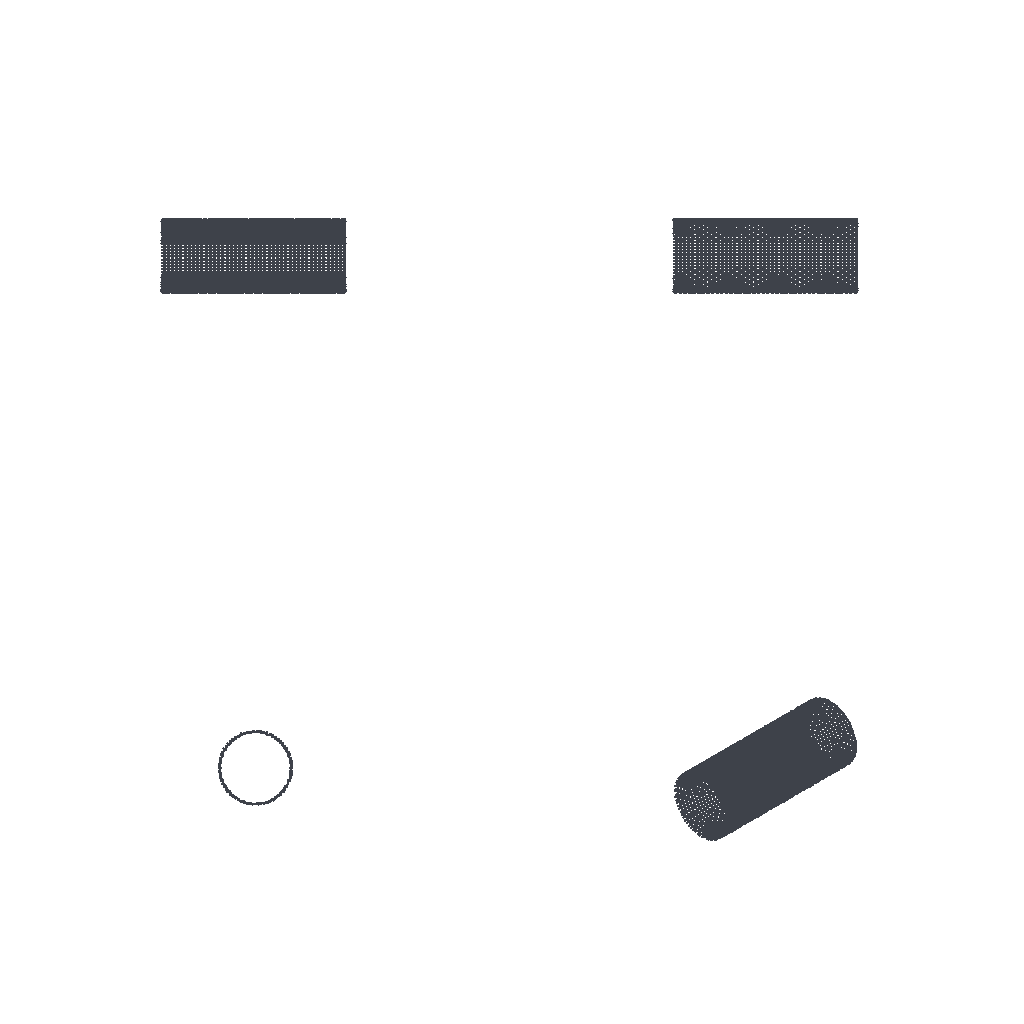Simulation study | abaqus
Set-up summary:
category,name,step,type,value,unit,region
solver,abaqus
solver,version,,,Abaqus/Explicit 2020
units,not stated in the deck,,not stated
analysis,deck,,transient,transient
load_step,Step-ya,Step-ya,transient,nlgeom=True
load_step,Step-1,Step-1,transient,nlgeom=True
contact,interactions,,,general=1 pairs=0 ties=0
load_step,requested,,,2
mesh,nodes,,,41311
mesh,elements,,,40572
element_type,R3D4,,rigid,12500
element_type,T3D2,,truss,28072
load,load commands in deck,,count,4
bc,support commands in deck,,count,26
material,MATERIAL-1,,in results
check,setup vs results,,match,"per instance, exact: element labels, types and connectivity; labels of the nodes the elements use; coordinates of those nodes at SINGLE_PRECISION in 116 of 116 instance(s)"
Abaqus input file, long lists of numbers shortened:
*Heading
** Job name: Job-3 Model name: Model-1-Copy-Copy
** Generated by: Abaqus/CAE 2020
*Preprint, echo=NO, model=NO, history=NO, contact=NO
**
** PARTS
**
*Part, name=jing-1
*Node
      1,         8.75,  0.2408,           0.
      2,        9.625,  0.2408,           0.
** (239 more lines like these left out)
*Element, type=T3D2
 1,  1, 22
 2, 22, 23
** (238 more lines like these left out)
*Nset, nset=Set-1, generate
   1,  241,    1
*Elset, elset=Set-1, generate
   1,  240,    1
** Section: Section-2
*Solid Section, elset=Set-1, material=Material-1
0.0045,
*End Part
**
*Part, name=jing-2
*Node
      1,   23.642,  0.2408,           0.
      2,   24.517,  0.2408,           0.
** (208 more lines like these left out)
*Element, type=T3D2
 1,  1, 31
 2, 31, 32
** (198 more lines like these left out)
*Nset, nset=Set-1, generate
   1,  210,    1
*Elset, elset=Set-1, generate
   1,  200,    1
** Section: Section-2
*Solid Section, elset=Set-1, material=Material-1
0.0045,
*End Part
**
*Part, name=qiao
*Node
      1,          25.,           0.,           0.
      2,   24.8,           0.,           0.
** (6424 more lines like these left out)
*Element, type=R3D4
   1,    1,    2,  128,  127
   2,    2,    3,  129,  128
** (6248 more lines like these left out)
*Node
   6427,         12.5,          -5.,           0.
*Nset, nset=qiao-RefPt_, internal
6427,
*Elset, elset=qiao, generate
    1,  6250,     1
*End Part
**
*Part, name=wei-1
*Node
      1,           0.,   3.803,           0.
      2, -0.5904,   3.752,           0.
** (286 more lines like these left out)
*Element, type=T3D2
1,  2, 37
2, 37, 38
** (286 more lines like these left out)
*Nset, nset=Set-1, generate
   1,  288,    1
*Elset, elset=Set-1, generate
   1,  288,    1
** Section: Section-1
*Solid Section, elset=Set-1, material=Material-1
0.003,
*End Part
**
**
** ASSEMBLY
**
*Assembly, name=Assembly
**
*Instance, name=jing-1-1, part=jing-1
          0.,          3.2,           0.
*End Instance
**
*Instance, name=jing-1-1-rad-2, part=jing-1
          0., 3.149, 0.5714
          0., 3.149, 0.5714, 1., 3.149, 0.5714, 10.286
*End Instance
**
*Instance, name=jing-1-1-rad-3, part=jing-1
          0., 2.996, 1.124
          0., 2.996, 1.124, 1., 2.996, 1.124, 20.571
*End Instance
**
*Instance, name=jing-1-1-rad-4, part=jing-1
          0., 2.747, 1.641
          0., 2.747, 1.641, 1., 2.747, 1.641, 30.857
*End Instance
**
*Instance, name=jing-1-1-rad-5, part=jing-1
          0., 2.41, 2.105
          0., 2.41, 2.105, 1., 2.41, 2.105, 41.143
*End Instance
**
*Instance, name=jing-1-1-rad-6, part=jing-1
          0., 1.995, 2.502
          0., 1.995, 2.502, 1., 1.995, 2.502, 51.429
*End Instance
**
*Instance, name=jing-1-1-rad-7, part=jing-1
          0., 1.516, 2.818
          0., 1.516, 2.818, 1., 1.516, 2.818, 61.714
*End Instance
**
*Instance, name=jing-1-1-rad-8, part=jing-1
          0., 0.9889, 3.043
          0., 0.9889, 3.043, 1., 0.9889, 3.043, 72.
*End Instance
**
*Instance, name=jing-1-1-rad-9, part=jing-1
          0., 0.4295, 3.171
          0., 0.4295, 3.171, 1., 0.4295, 3.171, 82.286
*End Instance
**
*Instance, name=jing-1-1-rad-10, part=jing-1
          0., -0.1436, 3.197
          0., -0.1436, 3.197, 1., -0.1436, 3.197, 92.571
*End Instance
**
*Instance, name=jing-1-1-rad-11, part=jing-1
          0., -0.7121, 3.12
          0., -0.7121, 3.12, 1., -0.7121, 3.12, 102.857
*End Instance
**
*Instance, name=jing-1-1-rad-12, part=jing-1
          0., -1.258, 2.942
          0., -1.258, 2.942, 1., -1.258, 2.942, 113.143
*End Instance
**
*Instance, name=jing-1-1-rad-13, part=jing-1
          0., -1.763, 2.671
          0., -1.763, 2.671, 1., -1.763, 2.671, 123.429
*End Instance
**
*Instance, name=jing-1-1-rad-14, part=jing-1
          0., -2.211, 2.313
          0., -2.211, 2.313, 1., -2.211, 2.313, 133.714
*End Instance
**
*Instance, name=jing-1-1-rad-15, part=jing-1
          0., -2.589, 1.881
          0., -2.589, 1.881, 1., -2.589, 1.881, 144.
*End Instance
**
*Instance, name=jing-1-1-rad-16, part=jing-1
          0., -2.883, 1.388
          0., -2.883, 1.388, 1., -2.883, 1.388, 154.286
*End Instance
**
*Instance, name=jing-1-1-rad-17, part=jing-1
          0., -3.085, 0.8513
          0., -3.085, 0.8513, 1., -3.085, 0.8513, 164.571
*End Instance
**
*Instance, name=jing-1-1-rad-18, part=jing-1
          0., -3.187, 0.2868
          0., -3.187, 0.2868, 1., -3.187, 0.2868, 174.857
*End Instance
**
*Instance, name=jing-1-1-rad-19, part=jing-1
          0., -3.187, -0.2868
          0., -3.187, -0.2868, 1., -3.187, -0.2868, 185.143
*End Instance
**
*Instance, name=jing-1-1-rad-20, part=jing-1
          0., -3.085, -0.8513
          0., -3.085, -0.8513, 1., -3.085, -0.8513, 195.429
*End Instance
**
*Instance, name=jing-1-1-rad-21, part=jing-1
          0., -2.883, -1.388
          0., -2.883, -1.388, 1., -2.883, -1.388, 205.714
*End Instance
**
*Instance, name=jing-1-1-rad-22, part=jing-1
          0., -2.589, -1.881
          0., -2.589, -1.881, 1., -2.589, -1.881, 216.
*End Instance
**
*Instance, name=jing-1-1-rad-23, part=jing-1
          0., -2.211, -2.313
          0., -2.211, -2.313, 1., -2.211, -2.313, 226.286
*End Instance
**
*Instance, name=jing-1-1-rad-24, part=jing-1
          0., -1.763, -2.671
          0., -1.763, -2.671, 1., -1.763, -2.671, 236.571
*End Instance
**
*Instance, name=jing-1-1-rad-25, part=jing-1
          0., -1.258, -2.942
          0., -1.258, -2.942, -1., -1.258, -2.942, 113.143
*End Instance
**
*Instance, name=jing-1-1-rad-26, part=jing-1
          0., -0.7121, -3.12
          0., -0.7121, -3.12, -1., -0.7121, -3.12, 102.857
*End Instance
**
*Instance, name=jing-1-1-rad-27, part=jing-1
          0., -0.1436, -3.197
          0., -0.1436, -3.197, -1., -0.1436, -3.197, 92.571
*End Instance
**
*Instance, name=jing-1-1-rad-28, part=jing-1
          0., 0.4295, -3.171
          0., 0.4295, -3.171, -1., 0.4295, -3.171, 82.286
*End Instance
**
*Instance, name=jing-1-1-rad-29, part=jing-1
          0., 0.9889, -3.043
          0., 0.9889, -3.043, -1., 0.9889, -3.043, 72.
*End Instance
**
*Instance, name=jing-1-1-rad-30, part=jing-1
          0., 1.516, -2.818
          0., 1.516, -2.818, -1., 1.516, -2.818, 61.714
*End Instance
**
*Instance, name=jing-1-1-rad-31, part=jing-1
          0., 1.995, -2.502
          0., 1.995, -2.502, -1., 1.995, -2.502, 51.429
*End Instance
**
*Instance, name=jing-1-1-rad-32, part=jing-1
          0., 2.41, -2.105
          0., 2.41, -2.105, -1., 2.41, -2.105, 41.143
*End Instance
**
*Instance, name=jing-1-1-rad-33, part=jing-1
          0., 2.747, -1.641
          0., 2.747, -1.641, -1., 2.747, -1.641, 30.857
*End Instance
**
*Instance, name=jing-1-1-rad-34, part=jing-1
          0., 2.996, -1.124
          0., 2.996, -1.124, -1., 2.996, -1.124, 20.571
*End Instance
**
*Instance, name=jing-1-1-rad-35, part=jing-1
          0., 3.149, -0.5714
          0., 3.149, -0.5714, -1., 3.149, -0.5714, 10.286
*End Instance
**
*Instance, name=jing-2-1, part=jing-2
          0., 3.188, 0.2789
          0., 3.188, 0.2789, 1., 3.188, 0.2789, 5.
*End Instance
**
*Instance, name=jing-2-1-rad-2, part=jing-2
          0., 3.087, 0.8436
          0., 3.087, 0.8436, 1., 3.087, 0.8436, 15.286
*End Instance
**
*Instance, name=jing-2-1-rad-3, part=jing-2
          0., 2.887, 1.381
          0., 2.887, 1.381, 1., 2.887, 1.381, 25.571
*End Instance
**
*Instance, name=jing-2-1-rad-4, part=jing-2
          0., 2.594, 1.874
          0., 2.594, 1.874, 1., 2.594, 1.874, 35.857
*End Instance
**
*Instance, name=jing-2-1-rad-5, part=jing-2
          0., 2.217, 2.307
          0., 2.217, 2.307, 1., 2.217, 2.307, 46.143
*End Instance
**
*Instance, name=jing-2-1-rad-6, part=jing-2
          0., 1.77, 2.666
          0., 1.77, 2.666, 1., 1.77, 2.666, 56.429
*End Instance
**
*Instance, name=jing-2-1-rad-7, part=jing-2
          0., 1.265, 2.939
          0., 1.265, 2.939, 1., 1.265, 2.939, 66.714
*End Instance
**
*Instance, name=jing-2-1-rad-8, part=jing-2
          0., 0.7198, 3.118
          0., 0.7198, 3.118, 1., 0.7198, 3.118, 77.
*End Instance
**
*Instance, name=jing-2-1-rad-9, part=jing-2
          0., 0.1515, 3.196
          0., 0.1515, 3.196, 1., 0.1515, 3.196, 87.286
*End Instance
**
*Instance, name=jing-2-1-rad-10, part=jing-2
          0., -0.4216, 3.172
          0., -0.4216, 3.172, 1., -0.4216, 3.172, 97.571
*End Instance
**
*Instance, name=jing-2-1-rad-11, part=jing-2
          0., -0.9813, 3.046
          0., -0.9813, 3.046, 1., -0.9813, 3.046, 107.857
*End Instance
**
*Instance, name=jing-2-1-rad-12, part=jing-2
          0., -1.509, 2.822
          0., -1.509, 2.822, 1., -1.509, 2.822, 118.143
*End Instance
**
*Instance, name=jing-2-1-rad-13, part=jing-2
          0., -1.989, 2.507
          0., -1.989, 2.507, 1., -1.989, 2.507, 128.429
*End Instance
**
*Instance, name=jing-2-1-rad-14, part=jing-2
          0., -2.405, 2.111
          0., -2.405, 2.111, 1., -2.405, 2.111, 138.714
*End Instance
**
*Instance, name=jing-2-1-rad-15, part=jing-2
          0., -2.743, 1.648
          0., -2.743, 1.648, 1., -2.743, 1.648, 149.
*End Instance
**
*Instance, name=jing-2-1-rad-16, part=jing-2
          0., -2.993, 1.132
          0., -2.993, 1.132, 1., -2.993, 1.132, 159.286
*End Instance
**
*Instance, name=jing-2-1-rad-17, part=jing-2
          0., -3.147, 0.5792
          0., -3.147, 0.5792, 1., -3.147, 0.5792, 169.571
*End Instance
**
*Instance, name=jing-2-1-rad-18, part=jing-2
          0., -3.2, 0.007979
          0., -3.2, 0.007979, 1., -3.2, 0.007979, 179.857
*End Instance
**
*Instance, name=jing-2-1-rad-19, part=jing-2
          0., -3.15, -0.5635
          0., -3.15, -0.5635, 1., -3.15, -0.5635, 190.143
*End Instance
**
*Instance, name=jing-2-1-rad-20, part=jing-2
          0., -2.999, -1.117
          0., -2.999, -1.117, 1., -2.999, -1.117, 200.429
*End Instance
**
*Instance, name=jing-2-1-rad-21, part=jing-2
          0., -2.751, -1.634
          0., -2.751, -1.634, 1., -2.751, -1.634, 210.714
*End Instance
**
*Instance, name=jing-2-1-rad-22, part=jing-2
          0., -2.415, -2.099
          0., -2.415, -2.099, 1., -2.415, -2.099, 221.
*End Instance
**
*Instance, name=jing-2-1-rad-23, part=jing-2
          0., -2.001, -2.497
          0., -2.001, -2.497, 1., -2.001, -2.497, 231.286
*End Instance
**
*Instance, name=jing-2-1-rad-24, part=jing-2
          0., -1.523, -2.814
          0., -1.523, -2.814, -1., -1.523, -2.814, 118.429
*End Instance
**
*Instance, name=jing-2-1-rad-25, part=jing-2
          0., -0.9964, -3.041
          0., -0.9964, -3.041, -1., -0.9964, -3.041, 108.143
*End Instance
**
*Instance, name=jing-2-1-rad-26, part=jing-2
          0., -0.4375, -3.17
          0., -0.4375, -3.17, -1., -0.4375, -3.17, 97.857
*End Instance
**
*Instance, name=jing-2-1-rad-27, part=jing-2
          0., 0.1356, -3.197
          0., 0.1356, -3.197, -1., 0.1356, -3.197, 87.571
*End Instance
**
*Instance, name=jing-2-1-rad-28, part=jing-2
          0., 0.7043, -3.122
          0., 0.7043, -3.122, -1., 0.7043, -3.122, 77.286
*End Instance
**
*Instance, name=jing-2-1-rad-29, part=jing-2
          0., 1.25, -2.946
          0., 1.25, -2.946, -1., 1.25, -2.946, 67.
*End Instance
**
*Instance, name=jing-2-1-rad-30, part=jing-2
          0., 1.756, -2.675
          0., 1.756, -2.675, -1., 1.756, -2.675, 56.714
*End Instance
**
*Instance, name=jing-2-1-rad-31, part=jing-2
          0., 2.206, -2.318
          0., 2.206, -2.318, -1., 2.206, -2.318, 46.429
*End Instance
**
*Instance, name=jing-2-1-rad-32, part=jing-2
          0., 2.584, -1.887
          0., 2.584, -1.887, -1., 2.584, -1.887, 36.143
*End Instance
**
*Instance, name=jing-2-1-rad-33, part=jing-2
          0., 2.88, -1.396
          0., 2.88, -1.396, -1., 2.88, -1.396, 25.857
*End Instance
**
*Instance, name=jing-2-1-rad-34, part=jing-2
          0., 3.083, -0.859
          0., 3.083, -0.859, -1., 3.083, -0.859, 15.571
*End Instance
**
*Instance, name=jing-2-1-rad-35, part=jing-2
          0., 3.186, -0.2948
          0., 3.186, -0.2948, -1., 3.186, -0.2948, 5.286
*End Instance
**
*Instance, name=wei-1-1, part=wei-1
          9., -0.3951, -0.06959
          9., -0.3951, -0.06959, 9.07, 0.6, 8.23284404274927e-07, 90.279
*End Instance
**
*Instance, name=wei-1-1-lin-2-1, part=wei-1
         9.4, -0.3951, -0.06959
         9.4, -0.3951, -0.06959, 9.47, 0.6, 8.23284404274927e-07, 90.279
*End Instance
**
*Instance, name=wei-1-1-lin-3-1, part=wei-1
         9.8, -0.3951, -0.06959
         9.8, -0.3951, -0.06959, 9.87, 0.6, 8.23284404274927e-07, 90.279
*End Instance
**
*Instance, name=wei-1-1-lin-4-1, part=wei-1
        10.2, -0.3951, -0.06959
        10.2, -0.3951, -0.06959, 10.27, 0.6, 8.23284404274927e-07, 90.279
*End Instance
**
*Instance, name=wei-1-1-lin-5-1, part=wei-1
        10.6, -0.3951, -0.06959
        10.6, -0.3951, -0.06959, 10.67, 0.6, 8.23284404274927e-07, 90.279
*End Instance
**
*Instance, name=wei-1-1-lin-6-1, part=wei-1
         11., -0.3951, -0.06959
         11., -0.3951, -0.06959, 11.07, 0.6, 8.23284404274927e-07, 90.279
*End Instance
**
*Instance, name=wei-1-1-lin-7-1, part=wei-1
        11.4, -0.3951, -0.06959
        11.4, -0.3951, -0.06959, 11.47, 0.6, 8.23284404274927e-07, 90.279
*End Instance
**
*Instance, name=wei-1-1-lin-8-1, part=wei-1
        11.8, -0.3951, -0.06959
        11.8, -0.3951, -0.06959, 11.87, 0.6, 8.23284404274927e-07, 90.279
*End Instance
**
*Instance, name=wei-1-1-lin-9-1, part=wei-1
        12.2, -0.3951, -0.06959
        12.2, -0.3951, -0.06959, 12.27, 0.6, 8.23284404274927e-07, 90.279
*End Instance
**
*Instance, name=wei-1-1-lin-10-1, part=wei-1
        12.6, -0.3951, -0.06959
        12.6, -0.3951, -0.06959, 12.67, 0.6, 8.23284404274927e-07, 90.279
*End Instance
**
*Instance, name=wei-1-1-lin-11-1, part=wei-1
         13., -0.3951, -0.06959
         13., -0.3951, -0.06959, 13.07, 0.6, 8.23284404274927e-07, 90.279
*End Instance
**
*Instance, name=wei-1-1-lin-12-1, part=wei-1
        13.4, -0.3951, -0.06959
        13.4, -0.3951, -0.06959, 13.47, 0.6, 8.23284404274927e-07, 90.279
*End Instance
**
*Instance, name=wei-1-1-lin-13-1, part=wei-1
        13.8, -0.3951, -0.06959
        13.8, -0.3951, -0.06959, 13.87, 0.6, 8.23284404274927e-07, 90.279
*End Instance
**
*Instance, name=wei-1-1-lin-14-1, part=wei-1
        14.2, -0.3951, -0.06959
        14.2, -0.3951, -0.06959, 14.27, 0.6, 8.23284404274927e-07, 90.279
*End Instance
**
*Instance, name=wei-1-1-lin-15-1, part=wei-1
        14.6, -0.3951, -0.06959
        14.6, -0.3951, -0.06959, 14.67, 0.6, 8.23284404274927e-07, 90.279
*End Instance
**
*Instance, name=wei-1-1-lin-16-1, part=wei-1
         15., -0.3951, -0.06959
         15., -0.3951, -0.06959, 15.07, 0.6, 8.23284404274927e-07, 90.279
*End Instance
**
*Instance, name=wei-1-1-lin-17-1, part=wei-1
        15.4, -0.3951, -0.06959
        15.4, -0.3951, -0.06959, 15.47, 0.6, 8.23284404274927e-07, 90.279
*End Instance
**
*Instance, name=wei-1-1-lin-18-1, part=wei-1
        15.8, -0.3951, -0.06959
        15.8, -0.3951, -0.06959, 15.87, 0.6, 8.23284404274927e-07, 90.279
*End Instance
**
*Instance, name=wei-1-1-lin-19-1, part=wei-1
        16.2, -0.3951, -0.06959
        16.2, -0.3951, -0.06959, 16.27, 0.6, 8.23284404274927e-07, 90.279
*End Instance
**
*Instance, name=wei-1-1-lin-20-1, part=wei-1
        16.6, -0.3951, -0.06959
        16.6, -0.3951, -0.06959, 16.67, 0.6, 8.23284404274927e-07, 90.279
*End Instance
**
*Instance, name=wei-1-1-lin-21-1, part=wei-1
         17., -0.3951, -0.06959
         17., -0.3951, -0.06959, 17.07, 0.6, 8.23284404274927e-07, 90.279
*End Instance
**
*Instance, name=wei-1-1-lin-22-1, part=wei-1
        17.4, -0.3951, -0.06959
        17.4, -0.3951, -0.06959, 17.47, 0.6, 8.23284404274927e-07, 90.279
*End Instance
**
*Instance, name=wei-1-1-lin-23-1, part=wei-1
        17.8, -0.3951, -0.06959
        17.8, -0.3951, -0.06959, 17.87, 0.6, 8.23284404274927e-07, 90.279
*End Instance
**
*Instance, name=wei-1-1-lin-24-1, part=wei-1
        18.2, -0.3951, -0.06959
        18.2, -0.3951, -0.06959, 18.27, 0.6, 8.23284404274927e-07, 90.279
*End Instance
**
*Instance, name=wei-1-1-lin-25-1, part=wei-1
        18.6, -0.3951, -0.06959
        18.6, -0.3951, -0.06959, 18.67, 0.6, 8.23284404274927e-07, 90.279
*End Instance
**
*Instance, name=wei-1-1-lin-26-1, part=wei-1
         19., -0.3951, -0.06959
         19., -0.3951, -0.06959, 19.07, 0.6, 8.23284404274927e-07, 90.279
*End Instance
**
*Instance, name=wei-1-1-lin-27-1, part=wei-1
        19.4, -0.3951, -0.06959
        19.4, -0.3951, -0.06959, 19.47, 0.6, 8.23284404274927e-07, 90.279
*End Instance
**
*Instance, name=wei-1-1-lin-28-1, part=wei-1
        19.8, -0.3951, -0.06959
        19.8, -0.3951, -0.06959, 19.87, 0.6, 8.23284404274927e-07, 90.279
*End Instance
**
*Instance, name=wei-1-1-lin-29-1, part=wei-1
        20.2, -0.3951, -0.06959
        20.2, -0.3951, -0.06959, 20.27, 0.6, 8.23284404274927e-07, 90.279
*End Instance
**
*Instance, name=wei-1-1-lin-30-1, part=wei-1
        20.6, -0.3951, -0.06959
        20.6, -0.3951, -0.06959, 20.67, 0.6, 8.23284404274927e-07, 90.279
*End Instance
**
*Instance, name=wei-1-1-lin-31-1, part=wei-1
         21., -0.3951, -0.06959
         21., -0.3951, -0.06959, 21.07, 0.6, 8.23284404274927e-07, 90.279
*End Instance
**
*Instance, name=wei-1-1-lin-32-1, part=wei-1
        21.4, -0.3951, -0.06959
        21.4, -0.3951, -0.06959, 21.47, 0.6, 8.23284404274927e-07, 90.279
*End Instance
**
*Instance, name=wei-1-1-lin-33-1, part=wei-1
        21.8, -0.3951, -0.06959
        21.8, -0.3951, -0.06959, 21.87, 0.6, 8.23284404274927e-07, 90.279
*End Instance
**
*Instance, name=wei-1-1-lin-34-1, part=wei-1
        22.2, -0.3951, -0.06959
        22.2, -0.3951, -0.06959, 22.27, 0.6, 8.23284404274927e-07, 90.279
*End Instance
**
*Instance, name=wei-1-1-lin-35-1, part=wei-1
        22.6, -0.3951, -0.06959
        22.6, -0.3951, -0.06959, 22.67, 0.6, 8.23284404274927e-07, 90.279
*End Instance
**
*Instance, name=wei-1-1-lin-36-1, part=wei-1
         23., -0.3951, -0.06959
         23., -0.3951, -0.06959, 23.07, 0.6, 8.23284404274927e-07, 90.279
*End Instance
**
*Instance, name=wei-1-1-lin-37-1, part=wei-1
        23.4, -0.3951, -0.06959
        23.4, -0.3951, -0.06959, 23.47, 0.6, 8.23284404274927e-07, 90.279
*End Instance
**
*Instance, name=wei-1-1-lin-38-1, part=wei-1
        23.8, -0.3951, -0.06959
        23.8, -0.3951, -0.06959, 23.87, 0.6, 8.23284404274927e-07, 90.279
*End Instance
**
*Instance, name=wei-1-1-lin-39-1, part=wei-1
        24.2, -0.3951, -0.06959
        24.2, -0.3951, -0.06959, 24.27, 0.6, 8.23284404274927e-07, 90.279
*End Instance
**
*Instance, name=wei-1-1-lin-40-1, part=wei-1
        24.6, -0.3951, -0.06959
        24.6, -0.3951, -0.06959, 24.67, 0.6, 8.23284404274927e-07, 90.279
*End Instance
**
*Instance, name=wei-1-1-lin-41-1, part=wei-1
         25., -0.3951, -0.06959
         25., -0.3951, -0.06959, 25.07, 0.6, 8.23284404274927e-07, 90.279
*End Instance
**
*Instance, name=wei-1-1-lin-42-1, part=wei-1
        25.4, -0.3951, -0.06959
        25.4, -0.3951, -0.06959, 25.47, 0.6, 8.23284404274927e-07, 90.279
*End Instance
**
*Instance, name=wei-1-1-lin-43-1, part=wei-1
        25.8, -0.3951, -0.06959
        25.8, -0.3951, -0.06959, 25.87, 0.6, 8.23284404274927e-07, 90.279
*End Instance
**
*Instance, name=wei-1-1-lin-44-1, part=wei-1
        26.2, -0.3951, -0.06959
        26.2, -0.3951, -0.06959, 26.27, 0.6, 8.23284404274927e-07, 90.279
*End Instance
**
*Instance, name=qiao-1, part=qiao
        5.25,     4.962,     3.56
*End Instance
**
*Instance, name=qiao-1-lin-2-1, part=qiao
        5.25,     4.962,    -3.59
*End Instance
**
*Nset, nset=Set-1, instance=jing-1-1
  20,  21, 231, 232, 233, 234, 235, 236, 237, 238, 239, 240, 241
*Nset, nset=Set-1, instance=jing-1-1-rad-2
  20,  21, 231, 232, 233, 234, 235, 236, 237, 238, 239, 240, 241
*Nset, nset=Set-1, instance=jing-1-1-rad-3
  20,  21, 231, 232, 233, 234, 235, 236, 237, 238, 239, 240, 241
*Nset, nset=Set-1, instance=jing-1-1-rad-5
  20,  21, 231, 232, 233, 234, 235, 236, 237, 238, 239, 240, 241
*Nset, nset=Set-1, instance=jing-1-1-rad-9
  20,  21, 231, 232, 233, 234, 235, 236, 237, 238, 239, 240, 241
*Nset, nset=Set-1, instance=jing-1-1-rad-25
  20,  21, 231, 232, 233, 234, 235, 236, 237, 238, 239, 240, 241
*Nset, nset=Set-1, instance=jing-2-1-rad-22
  29,  30, 202, 203, 204, 205, 206, 207, 208, 209, 210
*Nset, nset=Set-1, instance=jing-2-1-rad-6
  29,  30, 202, 203, 204, 205, 206, 207, 208, 209, 210
*Nset, nset=Set-1, instance=jing-1-1-rad-17
  20,  21, 231, 232, 233, 234, 235, 236, 237, 238, 239, 240, 241
*Nset, nset=Set-1, instance=jing-1-1-rad-33
  20,  21, 231, 232, 233, 234, 235, 236, 237, 238, 239, 240, 241
*Nset, nset=Set-1, instance=jing-2-1-rad-30
  29,  30, 202, 203, 204, 205, 206, 207, 208, 209, 210
*Nset, nset=Set-1, instance=jing-2-1-rad-14
  29,  30, 202, 203, 204, 205, 206, 207, 208, 209, 210
*Nset, nset=Set-1, instance=wei-1-1-lin-43-1, generate
   1,  288,    1
*Nset, nset=Set-1, instance=jing-1-1-rad-13
  20,  21, 231, 232, 233, 234, 235, 236, 237, 238, 239, 240, 241
*Nset, nset=Set-1, instance=jing-1-1-rad-29
  20,  21, 231, 232, 233, 234, 235, 236, 237, 238, 239, 240, 241
*Nset, nset=Set-1, instance=jing-2-1-rad-26
  29,  30, 202, 203, 204, 205, 206, 207, 208, 209, 210
*Nset, nset=Set-1, instance=jing-2-1-rad-10
  29,  30, 202, 203, 204, 205, 206, 207, 208, 209, 210
*Nset, nset=Set-1, instance=jing-1-1-rad-21
  20,  21, 231, 232, 233, 234, 235, 236, 237, 238, 239, 240, 241
*Nset, nset=Set-1, instance=jing-2-1-rad-2
  29,  30, 202, 203, 204, 205, 206, 207, 208, 209, 210
*Nset, nset=Set-1, instance=jing-2-1-rad-34
  29,  30, 202, 203, 204, 205, 206, 207, 208, 209, 210
*Nset, nset=Set-1, instance=jing-2-1-rad-18
  29,  30, 202, 203, 204, 205, 206, 207, 208, 209, 210
*Nset, nset=Set-1, instance=jing-1-1-rad-7
  20,  21, 231, 232, 233, 234, 235, 236, 237, 238, 239, 240, 241
*Nset, nset=Set-1, instance=jing-1-1-rad-11
  20,  21, 231, 232, 233, 234, 235, 236, 237, 238, 239, 240, 241
*Nset, nset=Set-1, instance=jing-1-1-rad-27
  20,  21, 231, 232, 233, 234, 235, 236, 237, 238, 239, 240, 241
*Nset, nset=Set-1, instance=jing-2-1-rad-24
  29,  30, 202, 203, 204, 205, 206, 207, 208, 209, 210
*Nset, nset=Set-1, instance=jing-2-1-rad-8
  29,  30, 202, 203, 204, 205, 206, 207, 208, 209, 210
*Nset, nset=Set-1, instance=jing-1-1-rad-19
  20,  21, 231, 232, 233, 234, 235, 236, 237, 238, 239, 240, 241
*Nset, nset=Set-1, instance=jing-1-1-rad-35
  20,  21, 231, 232, 233, 234, 235, 236, 237, 238, 239, 240, 241
*Nset, nset=Set-1, instance=jing-2-1-rad-32
  29,  30, 202, 203, 204, 205, 206, 207, 208, 209, 210
*Nset, nset=Set-1, instance=jing-2-1-rad-16
  29,  30, 202, 203, 204, 205, 206, 207, 208, 209, 210
*Nset, nset=Set-1, instance=jing-1-1-rad-15
  20,  21, 231, 232, 233, 234, 235, 236, 237, 238, 239, 240, 241
*Nset, nset=Set-1, instance=jing-1-1-rad-31
  20,  21, 231, 232, 233, 234, 235, 236, 237, 238, 239, 240, 241
*Nset, nset=Set-1, instance=jing-2-1-rad-28
  29,  30, 202, 203, 204, 205, 206, 207, 208, 209, 210
*Nset, nset=Set-1, instance=jing-2-1-rad-12
  29,  30, 202, 203, 204, 205, 206, 207, 208, 209, 210
*Nset, nset=Set-1, instance=jing-1-1-rad-23
  20,  21, 231, 232, 233, 234, 235, 236, 237, 238, 239, 240, 241
*Nset, nset=Set-1, instance=jing-2-1-rad-4
  29,  30, 202, 203, 204, 205, 206, 207, 208, 209, 210
*Nset, nset=Set-1, instance=jing-2-1-rad-20
  29,  30, 202, 203, 204, 205, 206, 207, 208, 209, 210
*Nset, nset=Set-1, instance=jing-1-1-rad-4
  20,  21, 231, 232, 233, 234, 235, 236, 237, 238, 239, 240, 241
*Nset, nset=Set-1, instance=jing-1-1-rad-6
  20,  21, 231, 232, 233, 234, 235, 236, 237, 238, 239, 240, 241
*Nset, nset=Set-1, instance=jing-1-1-rad-10
  20,  21, 231, 232, 233, 234, 235, 236, 237, 238, 239, 240, 241
*Nset, nset=Set-1, instance=jing-1-1-rad-26
  20,  21, 231, 232, 233, 234, 235, 236, 237, 238, 239, 240, 241
*Nset, nset=Set-1, instance=jing-2-1-rad-23
  29,  30, 202, 203, 204, 205, 206, 207, 208, 209, 210
*Nset, nset=Set-1, instance=jing-2-1-rad-7
  29,  30, 202, 203, 204, 205, 206, 207, 208, 209, 210
*Nset, nset=Set-1, instance=jing-1-1-rad-18
  20,  21, 231, 232, 233, 234, 235, 236, 237, 238, 239, 240, 241
*Nset, nset=Set-1, instance=jing-1-1-rad-34
  20,  21, 231, 232, 233, 234, 235, 236, 237, 238, 239, 240, 241
*Nset, nset=Set-1, instance=jing-2-1-rad-31
  29,  30, 202, 203, 204, 205, 206, 207, 208, 209, 210
*Nset, nset=Set-1, instance=jing-2-1-rad-15
  29,  30, 202, 203, 204, 205, 206, 207, 208, 209, 210
*Nset, nset=Set-1, instance=wei-1-1-lin-44-1, generate
   1,  288,    1
*Nset, nset=Set-1, instance=jing-1-1-rad-14
  20,  21, 231, 232, 233, 234, 235, 236, 237, 238, 239, 240, 241
*Nset, nset=Set-1, instance=jing-1-1-rad-30
  20,  21, 231, 232, 233, 234, 235, 236, 237, 238, 239, 240, 241
*Nset, nset=Set-1, instance=jing-2-1-rad-27
  29,  30, 202, 203, 204, 205, 206, 207, 208, 209, 210
*Nset, nset=Set-1, instance=jing-2-1-rad-11
  29,  30, 202, 203, 204, 205, 206, 207, 208, 209, 210
*Nset, nset=Set-1, instance=jing-1-1-rad-22
  20,  21, 231, 232, 233, 234, 235, 236, 237, 238, 239, 240, 241
*Nset, nset=Set-1, instance=jing-2-1-rad-3
  29,  30, 202, 203, 204, 205, 206, 207, 208, 209, 210
*Nset, nset=Set-1, instance=jing-2-1-rad-35
  29,  30, 202, 203, 204, 205, 206, 207, 208, 209, 210
*Nset, nset=Set-1, instance=jing-2-1-rad-19
  29,  30, 202, 203, 204, 205, 206, 207, 208, 209, 210
*Nset, nset=Set-1, instance=jing-1-1-rad-8
  20,  21, 231, 232, 233, 234, 235, 236, 237, 238, 239, 240, 241
*Nset, nset=Set-1, instance=jing-1-1-rad-12
  20,  21, 231, 232, 233, 234, 235, 236, 237, 238, 239, 240, 241
*Nset, nset=Set-1, instance=jing-1-1-rad-28
  20,  21, 231, 232, 233, 234, 235, 236, 237, 238, 239, 240, 241
*Nset, nset=Set-1, instance=jing-2-1-rad-25
  29,  30, 202, 203, 204, 205, 206, 207, 208, 209, 210
*Nset, nset=Set-1, instance=jing-2-1-rad-9
  29,  30, 202, 203, 204, 205, 206, 207, 208, 209, 210
*Nset, nset=Set-1, instance=jing-1-1-rad-20
  20,  21, 231, 232, 233, 234, 235, 236, 237, 238, 239, 240, 241
*Nset, nset=Set-1, instance=jing-2-1
  29,  30, 202, 203, 204, 205, 206, 207, 208, 209, 210
*Nset, nset=Set-1, instance=jing-2-1-rad-33
  29,  30, 202, 203, 204, 205, 206, 207, 208, 209, 210
*Nset, nset=Set-1, instance=jing-2-1-rad-17
  29,  30, 202, 203, 204, 205, 206, 207, 208, 209, 210
*Nset, nset=Set-1, instance=jing-1-1-rad-16
  20,  21, 231, 232, 233, 234, 235, 236, 237, 238, 239, 240, 241
*Nset, nset=Set-1, instance=jing-1-1-rad-32
  20,  21, 231, 232, 233, 234, 235, 236, 237, 238, 239, 240, 241
*Nset, nset=Set-1, instance=jing-2-1-rad-29
  29,  30, 202, 203, 204, 205, 206, 207, 208, 209, 210
*Nset, nset=Set-1, instance=jing-2-1-rad-13
  29,  30, 202, 203, 204, 205, 206, 207, 208, 209, 210
*Nset, nset=Set-1, instance=jing-1-1-rad-24
  20,  21, 231, 232, 233, 234, 235, 236, 237, 238, 239, 240, 241
*Nset, nset=Set-1, instance=jing-2-1-rad-5
  29,  30, 202, 203, 204, 205, 206, 207, 208, 209, 210
*Nset, nset=Set-1, instance=jing-2-1-rad-21
  29,  30, 202, 203, 204, 205, 206, 207, 208, 209, 210
*Elset, elset=Set-1, instance=jing-1-1, generate
 229,  240,    1
*Elset, elset=Set-1, instance=jing-1-1-rad-2, generate
 229,  240,    1
*Elset, elset=Set-1, instance=jing-1-1-rad-3, generate
 229,  240,    1
*Elset, elset=Set-1, instance=jing-1-1-rad-5, generate
 229,  240,    1
*Elset, elset=Set-1, instance=jing-1-1-rad-9, generate
 229,  240,    1
*Elset, elset=Set-1, instance=jing-1-1-rad-25, generate
 229,  240,    1
*Elset, elset=Set-1, instance=jing-2-1-rad-22, generate
 191,  200,    1
*Elset, elset=Set-1, instance=jing-2-1-rad-6, generate
 191,  200,    1
*Elset, elset=Set-1, instance=jing-1-1-rad-17, generate
 229,  240,    1
*Elset, elset=Set-1, instance=jing-1-1-rad-33, generate
 229,  240,    1
*Elset, elset=Set-1, instance=jing-2-1-rad-30, generate
 191,  200,    1
*Elset, elset=Set-1, instance=jing-2-1-rad-14, generate
 191,  200,    1
*Elset, elset=Set-1, instance=wei-1-1-lin-43-1, generate
   1,  288,    1
*Elset, elset=Set-1, instance=jing-1-1-rad-13, generate
 229,  240,    1
*Elset, elset=Set-1, instance=jing-1-1-rad-29, generate
 229,  240,    1
*Elset, elset=Set-1, instance=jing-2-1-rad-26, generate
 191,  200,    1
*Elset, elset=Set-1, instance=jing-2-1-rad-10, generate
 191,  200,    1
*Elset, elset=Set-1, instance=jing-1-1-rad-21, generate
 229,  240,    1
*Elset, elset=Set-1, instance=jing-2-1-rad-2, generate
 191,  200,    1
*Elset, elset=Set-1, instance=jing-2-1-rad-34, generate
 191,  200,    1
*Elset, elset=Set-1, instance=jing-2-1-rad-18, generate
 191,  200,    1
*Elset, elset=Set-1, instance=jing-1-1-rad-7, generate
 229,  240,    1
*Elset, elset=Set-1, instance=jing-1-1-rad-11, generate
 229,  240,    1
*Elset, elset=Set-1, instance=jing-1-1-rad-27, generate
 229,  240,    1
*Elset, elset=Set-1, instance=jing-2-1-rad-24, generate
 191,  200,    1
*Elset, elset=Set-1, instance=jing-2-1-rad-8, generate
 191,  200,    1
*Elset, elset=Set-1, instance=jing-1-1-rad-19, generate
 229,  240,    1
*Elset, elset=Set-1, instance=jing-1-1-rad-35, generate
 229,  240,    1
*Elset, elset=Set-1, instance=jing-2-1-rad-32, generate
 191,  200,    1
*Elset, elset=Set-1, instance=jing-2-1-rad-16, generate
 191,  200,    1
*Elset, elset=Set-1, instance=jing-1-1-rad-15, generate
 229,  240,    1
*Elset, elset=Set-1, instance=jing-1-1-rad-31, generate
 229,  240,    1
*Elset, elset=Set-1, instance=jing-2-1-rad-28, generate
 191,  200,    1
*Elset, elset=Set-1, instance=jing-2-1-rad-12, generate
 191,  200,    1
*Elset, elset=Set-1, instance=jing-1-1-rad-23, generate
 229,  240,    1
*Elset, elset=Set-1, instance=jing-2-1-rad-4, generate
 191,  200,    1
*Elset, elset=Set-1, instance=jing-2-1-rad-20, generate
 191,  200,    1
*Elset, elset=Set-1, instance=jing-1-1-rad-4, generate
 229,  240,    1
*Elset, elset=Set-1, instance=jing-1-1-rad-6, generate
 229,  240,    1
*Elset, elset=Set-1, instance=jing-1-1-rad-10, generate
 229,  240,    1
*Elset, elset=Set-1, instance=jing-1-1-rad-26, generate
 229,  240,    1
*Elset, elset=Set-1, instance=jing-2-1-rad-23, generate
 191,  200,    1
*Elset, elset=Set-1, instance=jing-2-1-rad-7, generate
 191,  200,    1
*Elset, elset=Set-1, instance=jing-1-1-rad-18, generate
 229,  240,    1
*Elset, elset=Set-1, instance=jing-1-1-rad-34, generate
 229,  240,    1
*Elset, elset=Set-1, instance=jing-2-1-rad-31, generate
 191,  200,    1
*Elset, elset=Set-1, instance=jing-2-1-rad-15, generate
 191,  200,    1
*Elset, elset=Set-1, instance=wei-1-1-lin-44-1, generate
   1,  288,    1
*Elset, elset=Set-1, instance=jing-1-1-rad-14, generate
 229,  240,    1
*Elset, elset=Set-1, instance=jing-1-1-rad-30, generate
 229,  240,    1
*Elset, elset=Set-1, instance=jing-2-1-rad-27, generate
 191,  200,    1
*Elset, elset=Set-1, instance=jing-2-1-rad-11, generate
 191,  200,    1
*Elset, elset=Set-1, instance=jing-1-1-rad-22, generate
 229,  240,    1
*Elset, elset=Set-1, instance=jing-2-1-rad-3, generate
 191,  200,    1
*Elset, elset=Set-1, instance=jing-2-1-rad-35, generate
 191,  200,    1
*Elset, elset=Set-1, instance=jing-2-1-rad-19, generate
 191,  200,    1
*Elset, elset=Set-1, instance=jing-1-1-rad-8, generate
 229,  240,    1
*Elset, elset=Set-1, instance=jing-1-1-rad-12, generate
 229,  240,    1
*Elset, elset=Set-1, instance=jing-1-1-rad-28, generate
 229,  240,    1
*Elset, elset=Set-1, instance=jing-2-1-rad-25, generate
 191,  200,    1
*Elset, elset=Set-1, instance=jing-2-1-rad-9, generate
 191,  200,    1
*Elset, elset=Set-1, instance=jing-1-1-rad-20, generate
 229,  240,    1
*Elset, elset=Set-1, instance=jing-2-1, generate
 191,  200,    1
*Elset, elset=Set-1, instance=jing-2-1-rad-33, generate
 191,  200,    1
*Elset, elset=Set-1, instance=jing-2-1-rad-17, generate
 191,  200,    1
*Elset, elset=Set-1, instance=jing-1-1-rad-16, generate
 229,  240,    1
*Elset, elset=Set-1, instance=jing-1-1-rad-32, generate
 229,  240,    1
*Elset, elset=Set-1, instance=jing-2-1-rad-29, generate
 191,  200,    1
*Elset, elset=Set-1, instance=jing-2-1-rad-13, generate
 191,  200,    1
*Elset, elset=Set-1, instance=jing-1-1-rad-24, generate
 229,  240,    1
*Elset, elset=Set-1, instance=jing-2-1-rad-5, generate
 191,  200,    1
*Elset, elset=Set-1, instance=jing-2-1-rad-21, generate
 191,  200,    1
*Nset, nset=Set-2, instance=jing-1-1
 1,
*Nset, nset=Set-2, instance=jing-1-1-rad-2
 1,
*Nset, nset=Set-2, instance=jing-1-1-rad-3
 1,
*Nset, nset=Set-2, instance=jing-1-1-rad-5
 1,
*Nset, nset=Set-2, instance=jing-1-1-rad-9
 1,
*Nset, nset=Set-2, instance=jing-1-1-rad-25
 1,
*Nset, nset=Set-2, instance=jing-2-1-rad-22
 11,
*Nset, nset=Set-2, instance=jing-2-1-rad-6
 11,
*Nset, nset=Set-2, instance=jing-1-1-rad-17
 1,
*Nset, nset=Set-2, instance=jing-1-1-rad-33
 1,
*Nset, nset=Set-2, instance=jing-2-1-rad-30
 11,
*Nset, nset=Set-2, instance=jing-2-1-rad-14
 11,
*Nset, nset=Set-2, instance=jing-1-1-rad-13
 1,
*Nset, nset=Set-2, instance=jing-1-1-rad-29
 1,
*Nset, nset=Set-2, instance=jing-2-1-rad-26
 11,
*Nset, nset=Set-2, instance=jing-2-1-rad-10
 11,
*Nset, nset=Set-2, instance=jing-1-1-rad-21
 1,
*Nset, nset=Set-2, instance=jing-2-1-rad-2
 11,
*Nset, nset=Set-2, instance=jing-2-1-rad-34
 11,
*Nset, nset=Set-2, instance=jing-2-1-rad-18
 11,
*Nset, nset=Set-2, instance=jing-1-1-rad-7
 1,
*Nset, nset=Set-2, instance=jing-1-1-rad-11
 1,
*Nset, nset=Set-2, instance=jing-1-1-rad-27
 1,
*Nset, nset=Set-2, instance=jing-2-1-rad-24
 11,
*Nset, nset=Set-2, instance=jing-2-1-rad-8
 11,
*Nset, nset=Set-2, instance=jing-1-1-rad-19
 1,
*Nset, nset=Set-2, instance=jing-1-1-rad-35
 1,
*Nset, nset=Set-2, instance=jing-2-1-rad-32
 11,
*Nset, nset=Set-2, instance=jing-2-1-rad-16
 11,
*Nset, nset=Set-2, instance=jing-1-1-rad-15
 1,
*Nset, nset=Set-2, instance=jing-1-1-rad-31
 1,
*Nset, nset=Set-2, instance=jing-2-1-rad-28
 11,
*Nset, nset=Set-2, instance=jing-2-1-rad-12
 11,
*Nset, nset=Set-2, instance=jing-1-1-rad-23
 1,
*Nset, nset=Set-2, instance=jing-2-1-rad-4
 11,
*Nset, nset=Set-2, instance=wei-1-1, generate
   1,  288,    1
*Nset, nset=Set-2, instance=jing-2-1-rad-20
 11,
*Nset, nset=Set-2, instance=jing-1-1-rad-4
 1,
*Nset, nset=Set-2, instance=jing-1-1-rad-6
 1,
*Nset, nset=Set-2, instance=jing-1-1-rad-10
 1,
*Nset, nset=Set-2, instance=jing-1-1-rad-26
 1,
*Nset, nset=Set-2, instance=jing-2-1-rad-23
 11,
*Nset, nset=Set-2, instance=jing-2-1-rad-7
 11,
*Nset, nset=Set-2, instance=jing-1-1-rad-18
 1,
*Nset, nset=Set-2, instance=jing-1-1-rad-34
 1,
*Nset, nset=Set-2, instance=jing-2-1-rad-31
 11,
*Nset, nset=Set-2, instance=jing-2-1-rad-15
 11,
*Nset, nset=Set-2, instance=jing-1-1-rad-14
 1,
*Nset, nset=Set-2, instance=jing-1-1-rad-30
 1,
*Nset, nset=Set-2, instance=jing-2-1-rad-27
 11,
*Nset, nset=Set-2, instance=jing-2-1-rad-11
 11,
*Nset, nset=Set-2, instance=jing-1-1-rad-22
 1,
*Nset, nset=Set-2, instance=jing-2-1-rad-3
 11,
*Nset, nset=Set-2, instance=jing-2-1-rad-35
 11,
*Nset, nset=Set-2, instance=jing-2-1-rad-19
 11,
*Nset, nset=Set-2, instance=jing-1-1-rad-8
 1,
*Nset, nset=Set-2, instance=jing-1-1-rad-12
 1,
*Nset, nset=Set-2, instance=jing-1-1-rad-28
 1,
*Nset, nset=Set-2, instance=jing-2-1-rad-25
 11,
*Nset, nset=Set-2, instance=jing-2-1-rad-9
 11,
*Nset, nset=Set-2, instance=jing-1-1-rad-20
 1,
*Nset, nset=Set-2, instance=jing-2-1
 11,
*Nset, nset=Set-2, instance=jing-2-1-rad-33
 11,
*Nset, nset=Set-2, instance=jing-2-1-rad-17
 11,
*Nset, nset=Set-2, instance=jing-1-1-rad-16
 1,
*Nset, nset=Set-2, instance=jing-1-1-rad-32
 1,
*Nset, nset=Set-2, instance=jing-2-1-rad-29
 11,
*Nset, nset=Set-2, instance=jing-2-1-rad-13
 11,
*Nset, nset=Set-2, instance=jing-1-1-rad-24
 1,
*Nset, nset=Set-2, instance=jing-2-1-rad-5
 11,
*Nset, nset=Set-2, instance=wei-1-1-lin-2-1, generate
   1,  288,    1
*Nset, nset=Set-2, instance=jing-2-1-rad-21
 11,
*Elset, elset=Set-2, instance=wei-1-1, generate
   1,  288,    1
*Elset, elset=Set-2, instance=wei-1-1-lin-2-1, generate
   1,  288,    1
*Nset, nset=Set-3, instance=qiao-1-lin-2-1
 6427,
*Nset, nset=Set-4, instance=qiao-1
 6427,
*Rigid Body, ref node=qiao-1.qiao-RefPt_, elset=qiao-1.qiao
*Rigid Body, ref node=qiao-1-lin-2-1.qiao-RefPt_, elset=qiao-1-lin-2-1.qiao
*End Assembly
*Amplitude, name=Amp-1
             0.,              0.,            0.01,              1.
*Amplitude, name=Amp-2
             0.,              0.,            0.01,              1.
**
** MATERIALS
**
*Material, name=Material-1
*Damage Initiation, criterion=DUCTILE
 0.01,0.,0.
*Damage Evolution, type=DISPLACEMENT
 0.0001,
*Density
 1e-09,
*Elastic
500., 0.35
*Plastic
15.,0.
**
** INTERACTION PROPERTIES
**
*Surface Interaction, name=IntProp-1
*Friction
 0.1,
*Surface Behavior, pressure-overclosure=HARD
** ----------------------------------------------------------------
**
** STEP: Step-ya
**
*Step, name=Step-ya, nlgeom=YES
*Dynamic, Explicit
, 0.01
*Bulk Viscosity
0.06, 1.2
**
** BOUNDARY CONDITIONS
**
** Name: [REDACTED] : Displacement/rotation angle
*Boundary, amplitude=Amp-2
Set-3, 1, 1
Set-3, 2, 2
Set-3, 3, 3, 3.25
Set-3, 4, 4
Set-3, 5, 5
Set-3, 6, 6
** Name: [REDACTED] : Displacement/rotation angle
*Boundary, amplitude=Amp-2
Set-4, 1, 1
Set-4, 2, 2
Set-4, 3, 3, -3.25
Set-4, 4, 4
Set-4, 5, 5
Set-4, 6, 6
**
** INTERACTIONS
**
** Interaction: Int-2
*Contact, op=NEW
*Contact Inclusions, ALL EXTERIOR
*Contact Property Assignment
 ,  , IntProp-1
**
** OUTPUT REQUESTS
**
*Restart, write, number interval=1, time marks=NO
**
** FIELD OUTPUT: F-Output-1
**
*Output, field, number interval=10
*Node Output
CF, RF, RM, RT, U, V
*Element Output, directions=YES
CTSHR, E, LE, MISES, MISESMAX, MISESONLY, NE, PE, PEEQ, PEEQMAX, PEEQT, PEMAG, PRESSONLY, S, SDEG, SEQUT
SF, SSAVG, TSHR, VEEQ
*Contact Output
CDISP, CFORCE, CSTRESS
*Output, history, frequency=0
*End Step
** ----------------------------------------------------------------
**
** STEP: Step-1
**
*Step, name=Step-1, nlgeom=YES
*Dynamic, Explicit
, 0.01
*Bulk Viscosity
0.06, 1.2
**
** BOUNDARY CONDITIONS
**
** Name: BC-2 Type: 位移/转角
*Boundary, amplitude=Amp-1
Set-2, 1, 1, -3.
Set-2, 2, 2
Set-2, 3, 3
Set-2, 4, 4
Set-2, 5, 5
Set-2, 6, 6
** Name: BC-2-u Type: 位移/转角
*Boundary, amplitude=Amp-2
Set-1, 1, 1, 3.
Set-1, 2, 2
Set-1, 3, 3
Set-1, 4, 4
Set-1, 5, 5
Set-1, 6, 6
** Name: [REDACTED] : Displacement/rotation angle
*Boundary, amplitude=Amp-2
Set-3, 3, 3
** Name: [REDACTED] : Displacement/rotation angle
*Boundary, amplitude=Amp-2
Set-4, 3, 3
**
** OUTPUT REQUESTS
**
*Restart, write, number interval=1, time marks=NO
**
** FIELD OUTPUT: F-Output-1
**
*Output, field, number interval=10
*Node Output
CF, RF, RM, RT, U, V
*Element Output, directions=YES
CTSHR, E, LE, MISES, MISESMAX, MISESONLY, NE, PE, PEEQ, PEEQMAX, PEEQT, PEMAG, PRESSONLY, S, SDEG, SEQUT
SF, SSAVG, STATUS, TSHR, VEEQ
*Contact Output
CDISP, CFORCE, CSTRESS
**
** HISTORY OUTPUT: H-Output-1
**
*Output, history, variable=PRESELECT
*End Step
Results summary:
result,step,Step-ya,completed,increments=125101 time=0.01/0.01
result,step,Step-1,completed,increments=125862 time=0.01/0.01
result,analysis,,,transient
result,last_loadstep,,,2
result,analysis steps,,count,2
result,primary field,,,U
result,reaction total,,FX,0.000184,model units
result,reaction total,,FY,-0.001538,model units
result,reaction total,,FZ,0.002979,model units